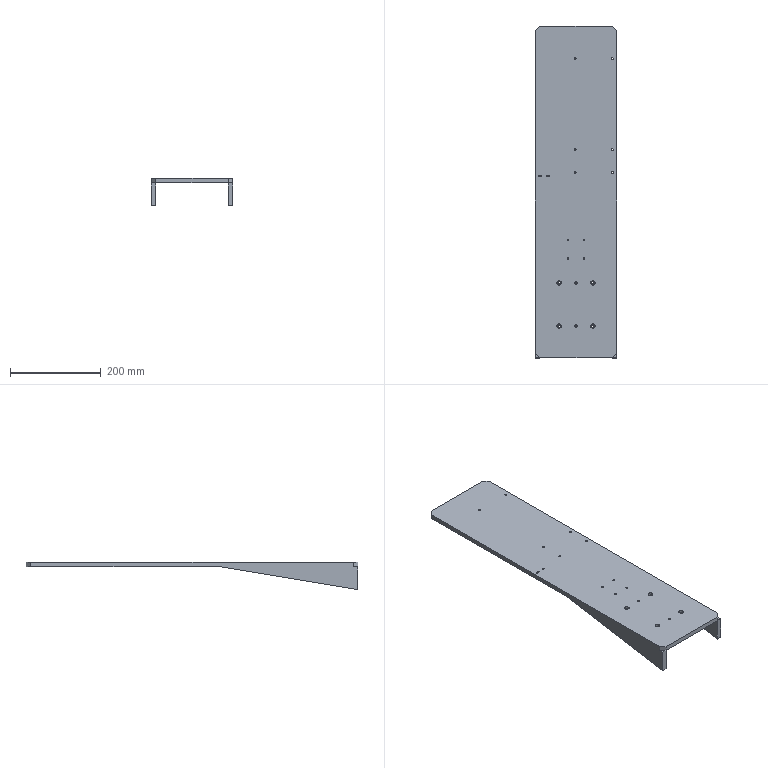Part | SolidWorks | features HoleWzd 5, Chamfer 1, Extrusion 1, ICE 1, MirrorPattern 1 | 1 solid | 70 faces | box 180 x 730 x 60 mm | volume 1457746 mm3 | cylinder 48 | plane 22 | commonest cylinder face diameters 4.2 x20 3.3 x8 5.5 x8 10 x8 5 x4